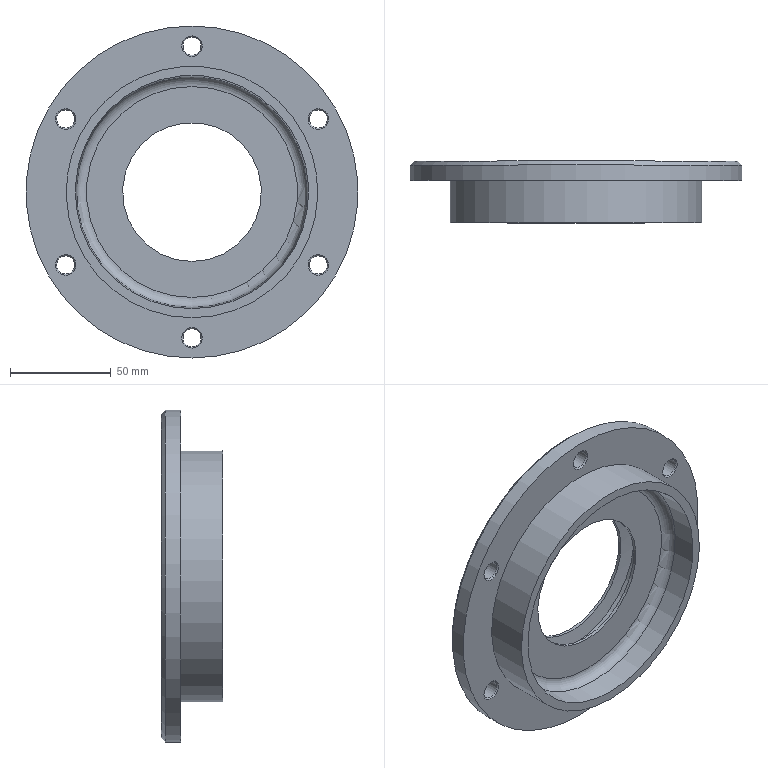Part | NX | 1 solid | 34 faces | box 165 x 30.6 x 165 mm | volume 204045 mm3 | cone 16 | cylinder 11 | plane 5 | torus 2 | commonest cylinder face diameters 9 x6 69 x2 85 x1 125 x1 165 x1
STEP:
#1=CARTESIAN_POINT('',(-58.89,28.801,-34.));
#2=VERTEX_POINT('',#1);
#3=CARTESIAN_POINT('',(-62.787,28.801,-36.25));
#4=DIRECTION('',(0.,-1.,0.));
#5=DIRECTION('',(0.866,0.,0.5));
#6=AXIS2_PLACEMENT_3D('',#3,#4,#5);
#7=CIRCLE('',#6,4.5);
#8=EDGE_CURVE('',#2,#2,#7,.T.);
#9=ORIENTED_EDGE('',*,*,#8,.F.);
#10=EDGE_LOOP('',(#9));
#11=FACE_BOUND('',#10,.T.);
#12=CARTESIAN_POINT('',(-58.37,28.201,-33.7));
#13=VERTEX_POINT('',#12);
#14=CARTESIAN_POINT('',(-62.787,28.201,-36.25));
#15=DIRECTION('',(0.,1.,0.));
#16=DIRECTION('',(0.866,0.,0.5));
#17=AXIS2_PLACEMENT_3D('',#14,#15,#16);
#18=CIRCLE('',#17,5.1);
#19=EDGE_CURVE('',#13,#13,#18,.T.);
#20=ORIENTED_EDGE('',*,*,#19,.F.);
#21=EDGE_LOOP('',(#20));
#22=FACE_BOUND('',#21,.T.);
#23=CARTESIAN_POINT('',(-62.787,28.201,-36.25));
#24=DIRECTION('',(0.,-1.,0.));
#25=DIRECTION('',(0.866,0.,0.5));
#26=AXIS2_PLACEMENT_3D('',#23,#24,#25);
#27=CONICAL_SURFACE('',#26,5.1,45.);
#28=ADVANCED_FACE('',(#11,#22),#27,.F.);
#29=CARTESIAN_POINT('',(-66.684,37.201,-38.5));
#30=VERTEX_POINT('',#29);
#31=CARTESIAN_POINT('',(-62.787,37.201,-36.25));
#32=DIRECTION('',(0.,1.,0.));
#33=DIRECTION('',(-0.866,0.,-0.5));
#34=AXIS2_PLACEMENT_3D('',#31,#32,#33);
#35=CIRCLE('',#34,4.5);
#36=EDGE_CURVE('',#30,#30,#35,.T.);
#37=ORIENTED_EDGE('',*,*,#36,.F.);
#38=EDGE_LOOP('',(#37));
#39=FACE_BOUND('',#38,.T.);
#40=CARTESIAN_POINT('',(-67.204,37.801,-38.8));
#41=VERTEX_POINT('',#40);
#42=CARTESIAN_POINT('',(-62.787,37.801,-36.25));
#43=DIRECTION('',(0.,-1.,0.));
#44=DIRECTION('',(-0.866,0.,-0.5));
#45=AXIS2_PLACEMENT_3D('',#42,#43,#44);
#46=CIRCLE('',#45,5.1);
#47=EDGE_CURVE('',#41,#41,#46,.T.);
#48=ORIENTED_EDGE('',*,*,#47,.F.);
#49=EDGE_LOOP('',(#48));
#50=FACE_BOUND('',#49,.T.);
#51=CARTESIAN_POINT('',(-62.787,37.801,-36.25));
#52=DIRECTION('',(0.,1.,0.));
#53=DIRECTION('',(-0.866,0.,-0.5));
#54=AXIS2_PLACEMENT_3D('',#51,#52,#53);
#55=CONICAL_SURFACE('',#54,5.1,45.);
#56=ADVANCED_FACE('',(#39,#50),#55,.F.);
#57=ORIENTED_EDGE('',*,*,#8,.T.);
#58=EDGE_LOOP('',(#57));
#59=FACE_BOUND('',#58,.T.);
#60=ORIENTED_EDGE('',*,*,#36,.T.);
#61=EDGE_LOOP('',(#60));
#62=FACE_BOUND('',#61,.T.);
#63=CARTESIAN_POINT('',(-62.787,37.801,-36.25));
#64=DIRECTION('',(0.,-1.,0.));
#65=DIRECTION('',(0.866,0.,0.5));
#66=AXIS2_PLACEMENT_3D('',#63,#64,#65);
#67=CYLINDRICAL_SURFACE('',#66,4.5);
#68=ADVANCED_FACE('',(#59,#62),#67,.F.);
#69=CARTESIAN_POINT('',(-58.89,28.801,34.));
#70=VERTEX_POINT('',#69);
#71=CARTESIAN_POINT('',(-62.787,28.801,36.25));
#72=DIRECTION('',(0.,-1.,0.));
#73=DIRECTION('',(0.866,0.,-0.5));
#74=AXIS2_PLACEMENT_3D('',#71,#72,#73);
#75=CIRCLE('',#74,4.5);
#76=EDGE_CURVE('',#70,#70,#75,.T.);
#77=ORIENTED_EDGE('',*,*,#76,.F.);
#78=EDGE_LOOP('',(#77));
#79=FACE_BOUND('',#78,.T.);
#80=CARTESIAN_POINT('',(-58.37,28.201,33.7));
#81=VERTEX_POINT('',#80);
#82=CARTESIAN_POINT('',(-62.787,28.201,36.25));
#83=DIRECTION('',(0.,1.,0.));
#84=DIRECTION('',(0.866,0.,-0.5));
#85=AXIS2_PLACEMENT_3D('',#82,#83,#84);
#86=CIRCLE('',#85,5.1);
#87=EDGE_CURVE('',#81,#81,#86,.T.);
#88=ORIENTED_EDGE('',*,*,#87,.F.);
#89=EDGE_LOOP('',(#88));
#90=FACE_BOUND('',#89,.T.);
#91=CARTESIAN_POINT('',(-62.787,28.201,36.25));
#92=DIRECTION('',(0.,-1.,0.));
#93=DIRECTION('',(0.866,0.,-0.5));
#94=AXIS2_PLACEMENT_3D('',#91,#92,#93);
#95=CONICAL_SURFACE('',#94,5.1,45.);
#96=ADVANCED_FACE('',(#79,#90),#95,.F.);
#97=CARTESIAN_POINT('',(-66.684,37.201,38.5));
#98=VERTEX_POINT('',#97);
#99=CARTESIAN_POINT('',(-62.787,37.201,36.25));
#100=DIRECTION('',(0.,1.,0.));
#101=DIRECTION('',(-0.866,0.,0.5));
#102=AXIS2_PLACEMENT_3D('',#99,#100,#101);
#103=CIRCLE('',#102,4.5);
#104=EDGE_CURVE('',#98,#98,#103,.T.);
#105=ORIENTED_EDGE('',*,*,#104,.F.);
#106=EDGE_LOOP('',(#105));
#107=FACE_BOUND('',#106,.T.);
#108=CARTESIAN_POINT('',(-67.204,37.801,38.8));
#109=VERTEX_POINT('',#108);
#110=CARTESIAN_POINT('',(-62.787,37.801,36.25));
#111=DIRECTION('',(0.,-1.,0.));
#112=DIRECTION('',(-0.866,0.,0.5));
#113=AXIS2_PLACEMENT_3D('',#110,#111,#112);
#114=CIRCLE('',#113,5.1);
#115=EDGE_CURVE('',#109,#109,#114,.T.);
#116=ORIENTED_EDGE('',*,*,#115,.F.);
#117=EDGE_LOOP('',(#116));
#118=FACE_BOUND('',#117,.T.);
#119=CARTESIAN_POINT('',(-62.787,37.801,36.25));
#120=DIRECTION('',(0.,1.,0.));
#121=DIRECTION('',(-0.866,0.,0.5));
#122=AXIS2_PLACEMENT_3D('',#119,#120,#121);
#123=CONICAL_SURFACE('',#122,5.1,45.);
#124=ADVANCED_FACE('',(#107,#118),#123,.F.);
#125=ORIENTED_EDGE('',*,*,#76,.T.);
#126=EDGE_LOOP('',(#125));
#127=FACE_BOUND('',#126,.T.);
#128=ORIENTED_EDGE('',*,*,#104,.T.);
#129=EDGE_LOOP('',(#128));
#130=FACE_BOUND('',#129,.T.);
#131=CARTESIAN_POINT('',(-62.787,37.801,36.25));
#132=DIRECTION('',(0.,-1.,0.));
#133=DIRECTION('',(0.866,0.,-0.5));
#134=AXIS2_PLACEMENT_3D('',#131,#132,#133);
#135=CYLINDRICAL_SURFACE('',#134,4.5);
#136=ADVANCED_FACE('',(#127,#130),#135,.F.);
#137=CARTESIAN_POINT('',(0.,28.801,68.));
#138=VERTEX_POINT('',#137);
#139=CARTESIAN_POINT('',(0.,28.801,72.5));
#140=DIRECTION('',(0.,-1.,0.));
#141=DIRECTION('',(0.,0.,-1.));
#142=AXIS2_PLACEMENT_3D('',#139,#140,#141);
#143=CIRCLE('',#142,4.5);
#144=EDGE_CURVE('',#138,#138,#143,.T.);
#145=ORIENTED_EDGE('',*,*,#144,.F.);
#146=EDGE_LOOP('',(#145));
#147=FACE_BOUND('',#146,.T.);
#148=CARTESIAN_POINT('',(0.,28.201,67.4));
#149=VERTEX_POINT('',#148);
#150=CARTESIAN_POINT('',(0.,28.201,72.5));
#151=DIRECTION('',(0.,1.,0.));
#152=DIRECTION('',(0.,0.,-1.));
#153=AXIS2_PLACEMENT_3D('',#150,#151,#152);
#154=CIRCLE('',#153,5.1);
#155=EDGE_CURVE('',#149,#149,#154,.T.);
#156=ORIENTED_EDGE('',*,*,#155,.F.);
#157=EDGE_LOOP('',(#156));
#158=FACE_BOUND('',#157,.T.);
#159=CARTESIAN_POINT('',(0.,28.201,72.5));
#160=DIRECTION('',(0.,-1.,0.));
#161=DIRECTION('',(0.,0.,-1.));
#162=AXIS2_PLACEMENT_3D('',#159,#160,#161);
#163=CONICAL_SURFACE('',#162,5.1,45.);
#164=ADVANCED_FACE('',(#147,#158),#163,.F.);
#165=CARTESIAN_POINT('',(0.,37.201,77.));
#166=VERTEX_POINT('',#165);
#167=CARTESIAN_POINT('',(0.,37.201,72.5));
#168=DIRECTION('',(0.,1.,0.));
#169=DIRECTION('',(0.,0.,1.));
#170=AXIS2_PLACEMENT_3D('',#167,#168,#169);
#171=CIRCLE('',#170,4.5);
#172=EDGE_CURVE('',#166,#166,#171,.T.);
#173=ORIENTED_EDGE('',*,*,#172,.F.);
#174=EDGE_LOOP('',(#173));
#175=FACE_BOUND('',#174,.T.);
#176=CARTESIAN_POINT('',(0.,37.801,77.6));
#177=VERTEX_POINT('',#176);
#178=CARTESIAN_POINT('',(0.,37.801,72.5));
#179=DIRECTION('',(0.,-1.,0.));
#180=DIRECTION('',(0.,0.,1.));
#181=AXIS2_PLACEMENT_3D('',#178,#179,#180);
#182=CIRCLE('',#181,5.1);
#183=EDGE_CURVE('',#177,#177,#182,.T.);
#184=ORIENTED_EDGE('',*,*,#183,.F.);
#185=EDGE_LOOP('',(#184));
#186=FACE_BOUND('',#185,.T.);
#187=CARTESIAN_POINT('',(0.,37.801,72.5));
#188=DIRECTION('',(0.,1.,0.));
#189=DIRECTION('',(0.,0.,1.));
#190=AXIS2_PLACEMENT_3D('',#187,#188,#189);
#191=CONICAL_SURFACE('',#190,5.1,45.);
#192=ADVANCED_FACE('',(#175,#186),#191,.F.);
#193=ORIENTED_EDGE('',*,*,#144,.T.);
#194=EDGE_LOOP('',(#193));
#195=FACE_BOUND('',#194,.T.);
#196=ORIENTED_EDGE('',*,*,#172,.T.);
#197=EDGE_LOOP('',(#196));
#198=FACE_BOUND('',#197,.T.);
#199=CARTESIAN_POINT('',(0.,37.801,72.5));
#200=DIRECTION('',(0.,-1.,0.));
#201=DIRECTION('',(0.,0.,-1.));
#202=AXIS2_PLACEMENT_3D('',#199,#200,#201);
#203=CYLINDRICAL_SURFACE('',#202,4.5);
#204=ADVANCED_FACE('',(#195,#198),#203,.F.);
#205=CARTESIAN_POINT('',(58.89,28.801,34.));
#206=VERTEX_POINT('',#205);
#207=CARTESIAN_POINT('',(62.787,28.801,36.25));
#208=DIRECTION('',(0.,-1.,0.));
#209=DIRECTION('',(-0.866,0.,-0.5));
#210=AXIS2_PLACEMENT_3D('',#207,#208,#209);
#211=CIRCLE('',#210,4.5);
#212=EDGE_CURVE('',#206,#206,#211,.T.);
#213=ORIENTED_EDGE('',*,*,#212,.F.);
#214=EDGE_LOOP('',(#213));
#215=FACE_BOUND('',#214,.T.);
#216=CARTESIAN_POINT('',(58.37,28.201,33.7));
#217=VERTEX_POINT('',#216);
#218=CARTESIAN_POINT('',(62.787,28.201,36.25));
#219=DIRECTION('',(0.,1.,0.));
#220=DIRECTION('',(-0.866,0.,-0.5));
#221=AXIS2_PLACEMENT_3D('',#218,#219,#220);
#222=CIRCLE('',#221,5.1);
#223=EDGE_CURVE('',#217,#217,#222,.T.);
#224=ORIENTED_EDGE('',*,*,#223,.F.);
#225=EDGE_LOOP('',(#224));
#226=FACE_BOUND('',#225,.T.);
#227=CARTESIAN_POINT('',(62.787,28.201,36.25));
#228=DIRECTION('',(0.,-1.,0.));
#229=DIRECTION('',(-0.866,0.,-0.5));
#230=AXIS2_PLACEMENT_3D('',#227,#228,#229);
#231=CONICAL_SURFACE('',#230,5.1,45.);
#232=ADVANCED_FACE('',(#215,#226),#231,.F.);
#233=CARTESIAN_POINT('',(66.684,37.201,38.5));
#234=VERTEX_POINT('',#233);
#235=CARTESIAN_POINT('',(62.787,37.201,36.25));
#236=DIRECTION('',(0.,1.,0.));
#237=DIRECTION('',(0.866,0.,0.5));
#238=AXIS2_PLACEMENT_3D('',#235,#236,#237);
#239=CIRCLE('',#238,4.5);
#240=EDGE_CURVE('',#234,#234,#239,.T.);
#241=ORIENTED_EDGE('',*,*,#240,.F.);
#242=EDGE_LOOP('',(#241));
#243=FACE_BOUND('',#242,.T.);
#244=CARTESIAN_POINT('',(67.204,37.801,38.8));
#245=VERTEX_POINT('',#244);
#246=CARTESIAN_POINT('',(62.787,37.801,36.25));
#247=DIRECTION('',(0.,-1.,0.));
#248=DIRECTION('',(0.866,0.,0.5));
#249=AXIS2_PLACEMENT_3D('',#246,#247,#248);
#250=CIRCLE('',#249,5.1);
#251=EDGE_CURVE('',#245,#245,#250,.T.);
#252=ORIENTED_EDGE('',*,*,#251,.F.);
#253=EDGE_LOOP('',(#252));
#254=FACE_BOUND('',#253,.T.);
#255=CARTESIAN_POINT('',(62.787,37.801,36.25));
#256=DIRECTION('',(0.,1.,0.));
#257=DIRECTION('',(0.866,0.,0.5));
#258=AXIS2_PLACEMENT_3D('',#255,#256,#257);
#259=CONICAL_SURFACE('',#258,5.1,45.);
#260=ADVANCED_FACE('',(#243,#254),#259,.F.);
#261=ORIENTED_EDGE('',*,*,#212,.T.);
#262=EDGE_LOOP('',(#261));
#263=FACE_BOUND('',#262,.T.);
#264=ORIENTED_EDGE('',*,*,#240,.T.);
#265=EDGE_LOOP('',(#264));
#266=FACE_BOUND('',#265,.T.);
#267=CARTESIAN_POINT('',(62.787,37.801,36.25));
#268=DIRECTION('',(0.,-1.,0.));
#269=DIRECTION('',(-0.866,0.,-0.5));
#270=AXIS2_PLACEMENT_3D('',#267,#268,#269);
#271=CYLINDRICAL_SURFACE('',#270,4.5);
#272=ADVANCED_FACE('',(#263,#266),#271,.F.);
#273=CARTESIAN_POINT('',(58.89,28.801,-34.));
#274=VERTEX_POINT('',#273);
#275=CARTESIAN_POINT('',(62.787,28.801,-36.25));
#276=DIRECTION('',(0.,-1.,0.));
#277=DIRECTION('',(-0.866,0.,0.5));
#278=AXIS2_PLACEMENT_3D('',#275,#276,#277);
#279=CIRCLE('',#278,4.5);
#280=EDGE_CURVE('',#274,#274,#279,.T.);
#281=ORIENTED_EDGE('',*,*,#280,.F.);
#282=EDGE_LOOP('',(#281));
#283=FACE_BOUND('',#282,.T.);
#284=CARTESIAN_POINT('',(58.37,28.201,-33.7));
#285=VERTEX_POINT('',#284);
#286=CARTESIAN_POINT('',(62.787,28.201,-36.25));
#287=DIRECTION('',(0.,1.,0.));
#288=DIRECTION('',(-0.866,0.,0.5));
#289=AXIS2_PLACEMENT_3D('',#286,#287,#288);
#290=CIRCLE('',#289,5.1);
#291=EDGE_CURVE('',#285,#285,#290,.T.);
#292=ORIENTED_EDGE('',*,*,#291,.F.);
#293=EDGE_LOOP('',(#292));
#294=FACE_BOUND('',#293,.T.);
#295=CARTESIAN_POINT('',(62.787,28.201,-36.25));
#296=DIRECTION('',(0.,-1.,0.));
#297=DIRECTION('',(-0.866,0.,0.5));
#298=AXIS2_PLACEMENT_3D('',#295,#296,#297);
#299=CONICAL_SURFACE('',#298,5.1,45.);
#300=ADVANCED_FACE('',(#283,#294),#299,.F.);
#301=CARTESIAN_POINT('',(66.684,37.201,-38.5));
#302=VERTEX_POINT('',#301);
#303=CARTESIAN_POINT('',(62.787,37.201,-36.25));
#304=DIRECTION('',(0.,1.,0.));
#305=DIRECTION('',(0.866,0.,-0.5));
#306=AXIS2_PLACEMENT_3D('',#303,#304,#305);
#307=CIRCLE('',#306,4.5);
#308=EDGE_CURVE('',#302,#302,#307,.T.);
#309=ORIENTED_EDGE('',*,*,#308,.F.);
#310=EDGE_LOOP('',(#309));
#311=FACE_BOUND('',#310,.T.);
#312=CARTESIAN_POINT('',(67.204,37.801,-38.8));
#313=VERTEX_POINT('',#312);
#314=CARTESIAN_POINT('',(62.787,37.801,-36.25));
#315=DIRECTION('',(0.,-1.,0.));
#316=DIRECTION('',(0.866,0.,-0.5));
#317=AXIS2_PLACEMENT_3D('',#314,#315,#316);
#318=CIRCLE('',#317,5.1);
#319=EDGE_CURVE('',#313,#313,#318,.T.);
#320=ORIENTED_EDGE('',*,*,#319,.F.);
#321=EDGE_LOOP('',(#320));
#322=FACE_BOUND('',#321,.T.);
#323=CARTESIAN_POINT('',(62.787,37.801,-36.25));
#324=DIRECTION('',(0.,1.,0.));
#325=DIRECTION('',(0.866,0.,-0.5));
#326=AXIS2_PLACEMENT_3D('',#323,#324,#325);
#327=CONICAL_SURFACE('',#326,5.1,45.);
#328=ADVANCED_FACE('',(#311,#322),#327,.F.);
#329=ORIENTED_EDGE('',*,*,#280,.T.);
#330=EDGE_LOOP('',(#329));
#331=FACE_BOUND('',#330,.T.);
#332=ORIENTED_EDGE('',*,*,#308,.T.);
#333=EDGE_LOOP('',(#332));
#334=FACE_BOUND('',#333,.T.);
#335=CARTESIAN_POINT('',(62.787,37.801,-36.25));
#336=DIRECTION('',(0.,-1.,0.));
#337=DIRECTION('',(-0.866,0.,0.5));
#338=AXIS2_PLACEMENT_3D('',#335,#336,#337);
#339=CYLINDRICAL_SURFACE('',#338,4.5);
#340=ADVANCED_FACE('',(#331,#334),#339,.F.);
#341=ORIENTED_EDGE('',*,*,#47,.T.);
#342=EDGE_LOOP('',(#341));
#343=FACE_BOUND('',#342,.T.);
#344=ORIENTED_EDGE('',*,*,#115,.T.);
#345=EDGE_LOOP('',(#344));
#346=FACE_BOUND('',#345,.T.);
#347=ORIENTED_EDGE('',*,*,#183,.T.);
#348=EDGE_LOOP('',(#347));
#349=FACE_BOUND('',#348,.T.);
#350=ORIENTED_EDGE('',*,*,#251,.T.);
#351=EDGE_LOOP('',(#350));
#352=FACE_BOUND('',#351,.T.);
#353=ORIENTED_EDGE('',*,*,#319,.T.);
#354=EDGE_LOOP('',(#353));
#355=FACE_BOUND('',#354,.T.);
#356=CARTESIAN_POINT('',(0.,37.801,-77.6));
#357=VERTEX_POINT('',#356);
#358=CARTESIAN_POINT('',(0.,37.801,-72.5));
#359=DIRECTION('',(0.,-1.,0.));
#360=DIRECTION('',(0.,0.,-1.));
#361=AXIS2_PLACEMENT_3D('',#358,#359,#360);
#362=CIRCLE('',#361,5.1);
#363=EDGE_CURVE('',#357,#357,#362,.T.);
#364=ORIENTED_EDGE('',*,*,#363,.T.);
#365=EDGE_LOOP('',(#364));
#366=FACE_BOUND('',#365,.T.);
#367=CARTESIAN_POINT('',(0.,37.801,-80.5));
#368=VERTEX_POINT('',#367);
#369=CARTESIAN_POINT('',(0.,37.801,0.));
#370=DIRECTION('',(0.,-1.,0.));
#371=DIRECTION('',(0.,0.,-1.));
#372=AXIS2_PLACEMENT_3D('',#369,#370,#371);
#373=CIRCLE('',#372,80.5);
#374=EDGE_CURVE('',#368,#368,#373,.T.);
#375=ORIENTED_EDGE('',*,*,#374,.F.);
#376=EDGE_LOOP('',(#375));
#377=FACE_BOUND('',#376,.T.);
#378=CARTESIAN_POINT('',(0.,37.801,-60.5));
#379=VERTEX_POINT('',#378);
#380=CARTESIAN_POINT('',(0.,37.801,0.));
#381=DIRECTION('',(0.,-1.,0.));
#382=DIRECTION('',(0.,0.,-1.));
#383=AXIS2_PLACEMENT_3D('',#380,#381,#382);
#384=CIRCLE('',#383,60.5);
#385=EDGE_CURVE('',#379,#379,#384,.T.);
#386=ORIENTED_EDGE('',*,*,#385,.T.);
#387=EDGE_LOOP('',(#386));
#388=FACE_BOUND('',#387,.T.);
#389=CARTESIAN_POINT('',(-60.5,37.801,0.));
#390=DIRECTION('',(0.,-1.,0.));
#391=DIRECTION('',(0.,0.,1.));
#392=AXIS2_PLACEMENT_3D('',#389,#390,#391);
#393=PLANE('',#392);
#394=ADVANCED_FACE('',(#343,#346,#349,#352,#355,#366,#377,#388),#393,.F.);
#395=CARTESIAN_POINT('',(0.,35.801,-82.5));
#396=VERTEX_POINT('',#395);
#397=CARTESIAN_POINT('',(0.,35.801,0.));
#398=DIRECTION('',(0.,-1.,0.));
#399=DIRECTION('',(0.,0.,-1.));
#400=AXIS2_PLACEMENT_3D('',#397,#398,#399);
#401=CIRCLE('',#400,82.5);
#402=EDGE_CURVE('',#396,#396,#401,.T.);
#403=ORIENTED_EDGE('',*,*,#402,.F.);
#404=EDGE_LOOP('',(#403));
#405=FACE_BOUND('',#404,.T.);
#406=ORIENTED_EDGE('',*,*,#374,.T.);
#407=EDGE_LOOP('',(#406));
#408=FACE_BOUND('',#407,.T.);
#409=CARTESIAN_POINT('',(0.,37.801,0.));
#410=DIRECTION('',(0.,-1.,0.));
#411=DIRECTION('',(0.,0.,1.));
#412=AXIS2_PLACEMENT_3D('',#409,#410,#411);
#413=CONICAL_SURFACE('',#412,80.5,45.);
#414=ADVANCED_FACE('',(#405,#408),#413,.T.);
#415=CARTESIAN_POINT('',(0.,28.201,-82.5));
#416=VERTEX_POINT('',#415);
#417=CARTESIAN_POINT('',(0.,28.201,0.));
#418=DIRECTION('',(0.,-1.,0.));
#419=DIRECTION('',(0.,0.,-1.));
#420=AXIS2_PLACEMENT_3D('',#417,#418,#419);
#421=CIRCLE('',#420,82.5);
#422=EDGE_CURVE('',#416,#416,#421,.T.);
#423=ORIENTED_EDGE('',*,*,#422,.F.);
#424=EDGE_LOOP('',(#423));
#425=FACE_BOUND('',#424,.T.);
#426=ORIENTED_EDGE('',*,*,#402,.T.);
#427=EDGE_LOOP('',(#426));
#428=FACE_BOUND('',#427,.T.);
#429=CARTESIAN_POINT('',(0.,63.971,0.));
#430=DIRECTION('',(0.,-1.,0.));
#431=DIRECTION('',(0.,0.,1.));
#432=AXIS2_PLACEMENT_3D('',#429,#430,#431);
#433=CYLINDRICAL_SURFACE('',#432,82.5);
#434=ADVANCED_FACE('',(#425,#428),#433,.T.);
#435=ORIENTED_EDGE('',*,*,#19,.T.);
#436=EDGE_LOOP('',(#435));
#437=FACE_BOUND('',#436,.T.);
#438=ORIENTED_EDGE('',*,*,#87,.T.);
#439=EDGE_LOOP('',(#438));
#440=FACE_BOUND('',#439,.T.);
#441=ORIENTED_EDGE('',*,*,#155,.T.);
#442=EDGE_LOOP('',(#441));
#443=FACE_BOUND('',#442,.T.);
#444=ORIENTED_EDGE('',*,*,#223,.T.);
#445=EDGE_LOOP('',(#444));
#446=FACE_BOUND('',#445,.T.);
#447=ORIENTED_EDGE('',*,*,#291,.T.);
#448=EDGE_LOOP('',(#447));
#449=FACE_BOUND('',#448,.T.);
#450=CARTESIAN_POINT('',(0.,28.201,-67.4));
#451=VERTEX_POINT('',#450);
#452=CARTESIAN_POINT('',(0.,28.201,-72.5));
#453=DIRECTION('',(0.,1.,0.));
#454=DIRECTION('',(0.,0.,1.));
#455=AXIS2_PLACEMENT_3D('',#452,#453,#454);
#456=CIRCLE('',#455,5.1);
#457=EDGE_CURVE('',#451,#451,#456,.T.);
#458=ORIENTED_EDGE('',*,*,#457,.T.);
#459=EDGE_LOOP('',(#458));
#460=FACE_BOUND('',#459,.T.);
#461=CARTESIAN_POINT('',(0.,28.201,-62.5));
#462=VERTEX_POINT('',#461);
#463=CARTESIAN_POINT('',(0.,28.201,0.));
#464=DIRECTION('',(0.,-1.,0.));
#465=DIRECTION('',(0.,0.,-1.));
#466=AXIS2_PLACEMENT_3D('',#463,#464,#465);
#467=CIRCLE('',#466,62.5);
#468=EDGE_CURVE('',#462,#462,#467,.T.);
#469=ORIENTED_EDGE('',*,*,#468,.F.);
#470=EDGE_LOOP('',(#469));
#471=FACE_BOUND('',#470,.T.);
#472=ORIENTED_EDGE('',*,*,#422,.T.);
#473=EDGE_LOOP('',(#472));
#474=FACE_BOUND('',#473,.T.);
#475=CARTESIAN_POINT('',(-82.5,28.201,0.));
#476=DIRECTION('',(0.,1.,0.));
#477=DIRECTION('',(0.,0.,-1.));
#478=AXIS2_PLACEMENT_3D('',#475,#476,#477);
#479=PLANE('',#478);
#480=ADVANCED_FACE('',(#437,#440,#443,#446,#449,#460,#471,#474),#479,.F.);
#481=CARTESIAN_POINT('',(0.,7.201,-62.5));
#482=VERTEX_POINT('',#481);
#483=CARTESIAN_POINT('',(0.,7.201,0.));
#484=DIRECTION('',(0.,-1.,0.));
#485=DIRECTION('',(0.,0.,-1.));
#486=AXIS2_PLACEMENT_3D('',#483,#484,#485);
#487=CIRCLE('',#486,62.5);
#488=EDGE_CURVE('',#482,#482,#487,.T.);
#489=ORIENTED_EDGE('',*,*,#488,.F.);
#490=EDGE_LOOP('',(#489));
#491=FACE_BOUND('',#490,.T.);
#492=ORIENTED_EDGE('',*,*,#468,.T.);
#493=EDGE_LOOP('',(#492));
#494=FACE_BOUND('',#493,.T.);
#495=CARTESIAN_POINT('',(0.,63.971,0.));
#496=DIRECTION('',(0.,-1.,0.));
#497=DIRECTION('',(0.,0.,1.));
#498=AXIS2_PLACEMENT_3D('',#495,#496,#497);
#499=CYLINDRICAL_SURFACE('',#498,62.5);
#500=ADVANCED_FACE('',(#491,#494),#499,.T.);
#501=CARTESIAN_POINT('',(0.,7.201,-58.));
#502=VERTEX_POINT('',#501);
#503=CARTESIAN_POINT('',(0.,7.201,0.));
#504=DIRECTION('',(0.,-1.,0.));
#505=DIRECTION('',(0.,0.,-1.));
#506=AXIS2_PLACEMENT_3D('',#503,#504,#505);
#507=CIRCLE('',#506,58.);
#508=EDGE_CURVE('',#502,#502,#507,.T.);
#509=ORIENTED_EDGE('',*,*,#508,.F.);
#510=EDGE_LOOP('',(#509));
#511=FACE_BOUND('',#510,.T.);
#512=ORIENTED_EDGE('',*,*,#488,.T.);
#513=EDGE_LOOP('',(#512));
#514=FACE_BOUND('',#513,.T.);
#515=CARTESIAN_POINT('',(-61.,7.201,0.));
#516=DIRECTION('',(0.,1.,0.));
#517=DIRECTION('',(0.,0.,-1.));
#518=AXIS2_PLACEMENT_3D('',#515,#516,#517);
#519=PLANE('',#518);
#520=ADVANCED_FACE('',(#511,#514),#519,.F.);
#521=CARTESIAN_POINT('',(0.,19.05,-57.408));
#522=VERTEX_POINT('',#521);
#523=CARTESIAN_POINT('',(0.,19.05,0.));
#524=DIRECTION('',(0.,-1.,0.));
#525=DIRECTION('',(0.,0.,-1.));
#526=AXIS2_PLACEMENT_3D('',#523,#524,#525);
#527=CIRCLE('',#526,57.408);
#528=EDGE_CURVE('',#522,#522,#527,.T.);
#529=ORIENTED_EDGE('',*,*,#528,.F.);
#530=EDGE_LOOP('',(#529));
#531=FACE_BOUND('',#530,.T.);
#532=ORIENTED_EDGE('',*,*,#508,.T.);
#533=EDGE_LOOP('',(#532));
#534=FACE_BOUND('',#533,.T.);
#535=CARTESIAN_POINT('',(0.,7.201,0.));
#536=DIRECTION('',(0.,-1.,0.));
#537=DIRECTION('',(0.,0.,1.));
#538=AXIS2_PLACEMENT_3D('',#535,#536,#537);
#539=CONICAL_SURFACE('',#538,58.,2.862);
#540=ADVANCED_FACE('',(#531,#534),#539,.F.);
#541=CARTESIAN_POINT('',(0.,23.801,-52.414));
#542=VERTEX_POINT('',#541);
#543=CARTESIAN_POINT('',(0.,23.801,0.));
#544=DIRECTION('',(0.,-1.,0.));
#545=DIRECTION('',(0.,0.,-1.));
#546=AXIS2_PLACEMENT_3D('',#543,#544,#545);
#547=CIRCLE('',#546,52.414);
#548=EDGE_CURVE('',#542,#542,#547,.T.);
#549=ORIENTED_EDGE('',*,*,#548,.F.);
#550=EDGE_LOOP('',(#549));
#551=FACE_BOUND('',#550,.T.);
#552=ORIENTED_EDGE('',*,*,#528,.T.);
#553=EDGE_LOOP('',(#552));
#554=FACE_BOUND('',#553,.T.);
#555=CARTESIAN_POINT('',(0.,18.801,0.));
#556=DIRECTION('',(0.,-1.,0.));
#557=DIRECTION('',(0.,0.,1.));
#558=AXIS2_PLACEMENT_3D('',#555,#556,#557);
#559=TOROIDAL_SURFACE('',#558,52.414,5.);
#560=ADVANCED_FACE('',(#551,#554),#559,.F.);
#561=CARTESIAN_POINT('',(0.,23.801,-34.5));
#562=VERTEX_POINT('',#561);
#563=CARTESIAN_POINT('',(0.,23.801,0.));
#564=DIRECTION('',(0.,-1.,0.));
#565=DIRECTION('',(0.,0.,-1.));
#566=AXIS2_PLACEMENT_3D('',#563,#564,#565);
#567=CIRCLE('',#566,34.5);
#568=EDGE_CURVE('',#562,#562,#567,.T.);
#569=ORIENTED_EDGE('',*,*,#568,.F.);
#570=EDGE_LOOP('',(#569));
#571=FACE_BOUND('',#570,.T.);
#572=ORIENTED_EDGE('',*,*,#548,.T.);
#573=EDGE_LOOP('',(#572));
#574=FACE_BOUND('',#573,.T.);
#575=CARTESIAN_POINT('',(-52.414,23.801,0.));
#576=DIRECTION('',(0.,1.,0.));
#577=DIRECTION('',(0.,0.,-1.));
#578=AXIS2_PLACEMENT_3D('',#575,#576,#577);
#579=PLANE('',#578);
#580=ADVANCED_FACE('',(#571,#574),#579,.F.);
#581=CARTESIAN_POINT('',(0.,25.318,-34.5));
#582=VERTEX_POINT('',#581);
#583=CARTESIAN_POINT('',(0.,25.318,0.));
#584=DIRECTION('',(0.,-1.,0.));
#585=DIRECTION('',(0.,0.,-1.));
#586=AXIS2_PLACEMENT_3D('',#583,#584,#585);
#587=CIRCLE('',#586,34.5);
#588=EDGE_CURVE('',#582,#582,#587,.T.);
#589=ORIENTED_EDGE('',*,*,#588,.F.);
#590=EDGE_LOOP('',(#589));
#591=FACE_BOUND('',#590,.T.);
#592=ORIENTED_EDGE('',*,*,#568,.T.);
#593=EDGE_LOOP('',(#592));
#594=FACE_BOUND('',#593,.T.);
#595=CARTESIAN_POINT('',(0.,63.971,0.));
#596=DIRECTION('',(0.,-1.,0.));
#597=DIRECTION('',(0.,0.,1.));
#598=AXIS2_PLACEMENT_3D('',#595,#596,#597);
#599=CYLINDRICAL_SURFACE('',#598,34.5);
#600=ADVANCED_FACE('',(#591,#594),#599,.F.);
#601=CARTESIAN_POINT('',(0.,26.301,-42.5));
#602=VERTEX_POINT('',#601);
#603=CARTESIAN_POINT('',(0.,26.301,0.));
#604=DIRECTION('',(0.,-1.,0.));
#605=DIRECTION('',(0.,0.,-1.));
#606=AXIS2_PLACEMENT_3D('',#603,#604,#605);
#607=CIRCLE('',#606,42.5);
#608=EDGE_CURVE('',#602,#602,#607,.T.);
#609=ORIENTED_EDGE('',*,*,#608,.F.);
#610=EDGE_LOOP('',(#609));
#611=FACE_BOUND('',#610,.T.);
#612=ORIENTED_EDGE('',*,*,#588,.T.);
#613=EDGE_LOOP('',(#612));
#614=FACE_BOUND('',#613,.T.);
#615=CARTESIAN_POINT('',(0.,25.318,0.));
#616=DIRECTION('',(0.,1.,0.));
#617=DIRECTION('',(0.,0.,-1.));
#618=AXIS2_PLACEMENT_3D('',#615,#616,#617);
#619=CONICAL_SURFACE('',#618,34.5,83.);
#620=ADVANCED_FACE('',(#611,#614),#619,.F.);
#621=CARTESIAN_POINT('',(0.,33.301,-42.5));
#622=VERTEX_POINT('',#621);
#623=CARTESIAN_POINT('',(0.,33.301,0.));
#624=DIRECTION('',(0.,-1.,0.));
#625=DIRECTION('',(0.,0.,-1.));
#626=AXIS2_PLACEMENT_3D('',#623,#624,#625);
#627=CIRCLE('',#626,42.5);
#628=EDGE_CURVE('',#622,#622,#627,.T.);
#629=ORIENTED_EDGE('',*,*,#628,.F.);
#630=EDGE_LOOP('',(#629));
#631=FACE_BOUND('',#630,.T.);
#632=ORIENTED_EDGE('',*,*,#608,.T.);
#633=EDGE_LOOP('',(#632));
#634=FACE_BOUND('',#633,.T.);
#635=CARTESIAN_POINT('',(0.,63.971,0.));
#636=DIRECTION('',(0.,-1.,0.));
#637=DIRECTION('',(0.,0.,1.));
#638=AXIS2_PLACEMENT_3D('',#635,#636,#637);
#639=CYLINDRICAL_SURFACE('',#638,42.5);
#640=ADVANCED_FACE('',(#631,#634),#639,.F.);
#641=CARTESIAN_POINT('',(0.,34.283,-34.5));
#642=VERTEX_POINT('',#641);
#643=CARTESIAN_POINT('',(0.,34.283,0.));
#644=DIRECTION('',(0.,-1.,0.));
#645=DIRECTION('',(0.,0.,-1.));
#646=AXIS2_PLACEMENT_3D('',#643,#644,#645);
#647=CIRCLE('',#646,34.5);
#648=EDGE_CURVE('',#642,#642,#647,.T.);
#649=ORIENTED_EDGE('',*,*,#648,.F.);
#650=EDGE_LOOP('',(#649));
#651=FACE_BOUND('',#650,.T.);
#652=ORIENTED_EDGE('',*,*,#628,.T.);
#653=EDGE_LOOP('',(#652));
#654=FACE_BOUND('',#653,.T.);
#655=CARTESIAN_POINT('',(0.,33.301,0.));
#656=DIRECTION('',(0.,-1.,0.));
#657=DIRECTION('',(0.,0.,1.));
#658=AXIS2_PLACEMENT_3D('',#655,#656,#657);
#659=CONICAL_SURFACE('',#658,42.5,83.);
#660=ADVANCED_FACE('',(#651,#654),#659,.F.);
#661=CARTESIAN_POINT('',(0.,35.801,-34.5));
#662=VERTEX_POINT('',#661);
#663=CARTESIAN_POINT('',(0.,35.801,0.));
#664=DIRECTION('',(0.,-1.,0.));
#665=DIRECTION('',(0.,0.,-1.));
#666=AXIS2_PLACEMENT_3D('',#663,#664,#665);
#667=CIRCLE('',#666,34.5);
#668=EDGE_CURVE('',#662,#662,#667,.T.);
#669=ORIENTED_EDGE('',*,*,#668,.F.);
#670=EDGE_LOOP('',(#669));
#671=FACE_BOUND('',#670,.T.);
#672=ORIENTED_EDGE('',*,*,#648,.T.);
#673=EDGE_LOOP('',(#672));
#674=FACE_BOUND('',#673,.T.);
#675=CARTESIAN_POINT('',(0.,63.971,0.));
#676=DIRECTION('',(0.,-1.,0.));
#677=DIRECTION('',(0.,0.,1.));
#678=AXIS2_PLACEMENT_3D('',#675,#676,#677);
#679=CYLINDRICAL_SURFACE('',#678,34.5);
#680=ADVANCED_FACE('',(#671,#674),#679,.F.);
#681=CARTESIAN_POINT('',(0.,35.801,-58.5));
#682=VERTEX_POINT('',#681);
#683=CARTESIAN_POINT('',(0.,35.801,0.));
#684=DIRECTION('',(0.,-1.,0.));
#685=DIRECTION('',(0.,0.,-1.));
#686=AXIS2_PLACEMENT_3D('',#683,#684,#685);
#687=CIRCLE('',#686,58.5);
#688=EDGE_CURVE('',#682,#682,#687,.T.);
#689=ORIENTED_EDGE('',*,*,#688,.F.);
#690=EDGE_LOOP('',(#689));
#691=FACE_BOUND('',#690,.T.);
#692=ORIENTED_EDGE('',*,*,#668,.T.);
#693=EDGE_LOOP('',(#692));
#694=FACE_BOUND('',#693,.T.);
#695=CARTESIAN_POINT('',(-34.5,35.801,0.));
#696=DIRECTION('',(0.,-1.,0.));
#697=DIRECTION('',(0.,0.,1.));
#698=AXIS2_PLACEMENT_3D('',#695,#696,#697);
#699=PLANE('',#698);
#700=ADVANCED_FACE('',(#691,#694),#699,.F.);
#701=ORIENTED_EDGE('',*,*,#385,.F.);
#702=EDGE_LOOP('',(#701));
#703=FACE_BOUND('',#702,.T.);
#704=ORIENTED_EDGE('',*,*,#688,.T.);
#705=EDGE_LOOP('',(#704));
#706=FACE_BOUND('',#705,.T.);
#707=CARTESIAN_POINT('',(0.,37.801,0.));
#708=DIRECTION('',(0.,-1.,0.));
#709=DIRECTION('',(0.,0.,1.));
#710=AXIS2_PLACEMENT_3D('',#707,#708,#709);
#711=TOROIDAL_SURFACE('',#710,58.5,2.);
#712=ADVANCED_FACE('',(#703,#706),#711,.F.);
#713=CARTESIAN_POINT('',(0.,28.801,-68.));
#714=VERTEX_POINT('',#713);
#715=CARTESIAN_POINT('',(0.,28.801,-72.5));
#716=DIRECTION('',(0.,-1.,0.));
#717=DIRECTION('',(0.,0.,1.));
#718=AXIS2_PLACEMENT_3D('',#715,#716,#717);
#719=CIRCLE('',#718,4.5);
#720=EDGE_CURVE('',#714,#714,#719,.T.);
#721=ORIENTED_EDGE('',*,*,#720,.T.);
#722=EDGE_LOOP('',(#721));
#723=FACE_BOUND('',#722,.T.);
#724=CARTESIAN_POINT('',(0.,37.201,-77.));
#725=VERTEX_POINT('',#724);
#726=CARTESIAN_POINT('',(0.,37.201,-72.5));
#727=DIRECTION('',(0.,1.,0.));
#728=DIRECTION('',(0.,0.,-1.));
#729=AXIS2_PLACEMENT_3D('',#726,#727,#728);
#730=CIRCLE('',#729,4.5);
#731=EDGE_CURVE('',#725,#725,#730,.T.);
#732=ORIENTED_EDGE('',*,*,#731,.T.);
#733=EDGE_LOOP('',(#732));
#734=FACE_BOUND('',#733,.T.);
#735=CARTESIAN_POINT('',(0.,37.801,-72.5));
#736=DIRECTION('',(0.,-1.,0.));
#737=DIRECTION('',(0.,0.,1.));
#738=AXIS2_PLACEMENT_3D('',#735,#736,#737);
#739=CYLINDRICAL_SURFACE('',#738,4.5);
#740=ADVANCED_FACE('',(#723,#734),#739,.F.);
#741=ORIENTED_EDGE('',*,*,#731,.F.);
#742=EDGE_LOOP('',(#741));
#743=FACE_BOUND('',#742,.T.);
#744=ORIENTED_EDGE('',*,*,#363,.F.);
#745=EDGE_LOOP('',(#744));
#746=FACE_BOUND('',#745,.T.);
#747=CARTESIAN_POINT('',(0.,37.801,-72.5));
#748=DIRECTION('',(0.,1.,0.));
#749=DIRECTION('',(0.,0.,-1.));
#750=AXIS2_PLACEMENT_3D('',#747,#748,#749);
#751=CONICAL_SURFACE('',#750,5.1,45.);
#752=ADVANCED_FACE('',(#743,#746),#751,.F.);
#753=ORIENTED_EDGE('',*,*,#720,.F.);
#754=EDGE_LOOP('',(#753));
#755=FACE_BOUND('',#754,.T.);
#756=ORIENTED_EDGE('',*,*,#457,.F.);
#757=EDGE_LOOP('',(#756));
#758=FACE_BOUND('',#757,.T.);
#759=CARTESIAN_POINT('',(0.,28.201,-72.5));
#760=DIRECTION('',(0.,-1.,0.));
#761=DIRECTION('',(0.,0.,1.));
#762=AXIS2_PLACEMENT_3D('',#759,#760,#761);
#763=CONICAL_SURFACE('',#762,5.1,45.);
#764=ADVANCED_FACE('',(#755,#758),#763,.F.);
#765=CLOSED_SHELL('',(#28,#56,#68,#96,#124,#136,#164,#192,#204,#232,#260,#272,#300,#328,#340,#394,#414,#434,#480,#500,#520,#540,#560,#580,#600,#620,#640,#660,#680,#700,#712,#740,#752,#764));
#766=MANIFOLD_SOLID_BREP('',#765);
#767=(LENGTH_UNIT()NAMED_UNIT(*)SI_UNIT(.MILLI.,.METRE.));
#768=UNCERTAINTY_MEASURE_WITH_UNIT(LENGTH_MEASURE(0.00002),#767,'','');
#769=(NAMED_UNIT(*)PLANE_ANGLE_UNIT()SI_UNIT($,.RADIAN.));
#770=PLANE_ANGLE_MEASURE_WITH_UNIT(PLANE_ANGLE_MEASURE(0.01745),#769);
#771=DIMENSIONAL_EXPONENTS(0.,0.,0.,0.,0.,0.,0.);
#772=(CONVERSION_BASED_UNIT('DEGREE',#770)NAMED_UNIT(#771)PLANE_ANGLE_UNIT());
#773=(NAMED_UNIT(*)SI_UNIT($,.STERADIAN.)SOLID_ANGLE_UNIT());
#774=(GEOMETRIC_REPRESENTATION_CONTEXT(3)GLOBAL_UNCERTAINTY_ASSIGNED_CONTEXT((#768))GLOBAL_UNIT_ASSIGNED_CONTEXT((#767,#772,#773))REPRESENTATION_CONTEXT('',''));
#775=ADVANCED_BREP_SHAPE_REPRESENTATION('',(#766),#774);